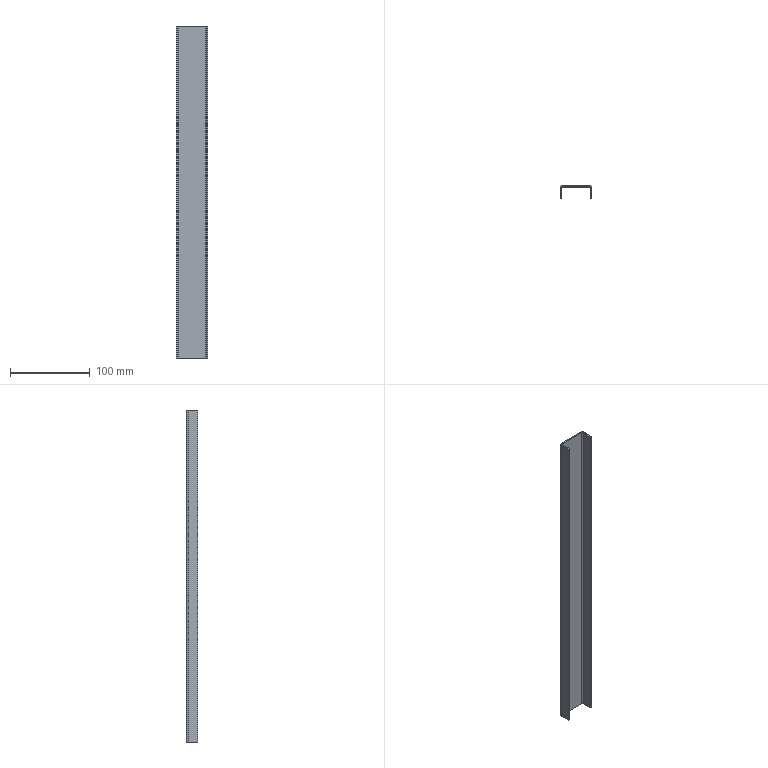Part | SolidWorks | features FlatPattern 1, SMBaseFlange 1, SheetMetal 1 | 1 solid | 22 faces | box 40 x 15 x 416 mm | volume 40603 mm3 | plane 18 | cylinder 4 | commonest cylinder face diameters 3 x2 6 x2
STEP:
#1=CARTESIAN_POINT('',(3.,15.,416.));
#2=VERTEX_POINT('',#1);
#3=CARTESIAN_POINT('',(3.,13.5,416.));
#4=VERTEX_POINT('',#3);
#5=CARTESIAN_POINT('',(3.,15.,416.));
#6=DIRECTION('',(0.,-1.,0.));
#7=VECTOR('',#6,1000.);
#8=LINE('',#5,#7);
#9=EDGE_CURVE('',#2,#4,#8,.T.);
#10=ORIENTED_EDGE('',*,*,#9,.F.);
#11=CARTESIAN_POINT('',(0.,12.,416.));
#12=VERTEX_POINT('',#11);
#13=CARTESIAN_POINT('',(3.,12.,416.));
#14=DIRECTION('',(0.,0.,-1.));
#15=DIRECTION('',(1.,0.,0.));
#16=AXIS2_PLACEMENT_3D('',#13,#14,#15);
#17=CIRCLE('',#16,3.);
#18=EDGE_CURVE('',#12,#2,#17,.T.);
#19=ORIENTED_EDGE('',*,*,#18,.F.);
#20=CARTESIAN_POINT('',(1.5,12.,416.));
#21=VERTEX_POINT('',#20);
#22=CARTESIAN_POINT('',(1.5,12.,416.));
#23=DIRECTION('',(-1.,0.,0.));
#24=VECTOR('',#23,1000.);
#25=LINE('',#22,#24);
#26=EDGE_CURVE('',#21,#12,#25,.T.);
#27=ORIENTED_EDGE('',*,*,#26,.F.);
#28=CARTESIAN_POINT('',(3.,12.,416.));
#29=DIRECTION('',(0.,0.,-1.));
#30=DIRECTION('',(1.,0.,0.));
#31=AXIS2_PLACEMENT_3D('',#28,#29,#30);
#32=CIRCLE('',#31,1.5);
#33=EDGE_CURVE('',#21,#4,#32,.T.);
#34=ORIENTED_EDGE('',*,*,#33,.T.);
#35=EDGE_LOOP('',(#10,#19,#27,#34));
#36=FACE_OUTER_BOUND('',#35,.T.);
#37=CARTESIAN_POINT('',(3.,15.,416.));
#38=DIRECTION('',(0.,0.,1.));
#39=DIRECTION('',(1.,0.,0.));
#40=AXIS2_PLACEMENT_3D('',#37,#38,#39);
#41=PLANE('',#40);
#42=ADVANCED_FACE('',(#36),#41,.T.);
#43=CARTESIAN_POINT('',(37.,15.,416.));
#44=VERTEX_POINT('',#43);
#45=CARTESIAN_POINT('',(0.,15.,416.));
#46=DIRECTION('',(1.,0.,0.));
#47=VECTOR('',#46,1000.);
#48=LINE('',#45,#47);
#49=EDGE_CURVE('',#2,#44,#48,.T.);
#50=ORIENTED_EDGE('',*,*,#49,.F.);
#51=ORIENTED_EDGE('',*,*,#9,.T.);
#52=CARTESIAN_POINT('',(37.,13.5,416.));
#53=VERTEX_POINT('',#52);
#54=CARTESIAN_POINT('',(0.,13.5,416.));
#55=DIRECTION('',(1.,0.,0.));
#56=VECTOR('',#55,1000.);
#57=LINE('',#54,#56);
#58=EDGE_CURVE('',#4,#53,#57,.T.);
#59=ORIENTED_EDGE('',*,*,#58,.T.);
#60=CARTESIAN_POINT('',(37.,13.5,416.));
#61=DIRECTION('',(0.,1.,0.));
#62=VECTOR('',#61,1000.);
#63=LINE('',#60,#62);
#64=EDGE_CURVE('',#53,#44,#63,.T.);
#65=ORIENTED_EDGE('',*,*,#64,.T.);
#66=EDGE_LOOP('',(#50,#51,#59,#65));
#67=FACE_OUTER_BOUND('',#66,.T.);
#68=CARTESIAN_POINT('',(1.5,12.,416.));
#69=DIRECTION('',(0.,0.,1.));
#70=DIRECTION('',(1.,0.,0.));
#71=AXIS2_PLACEMENT_3D('',#68,#69,#70);
#72=PLANE('',#71);
#73=ADVANCED_FACE('',(#67),#72,.T.);
#74=CARTESIAN_POINT('',(0.,12.,0.));
#75=VERTEX_POINT('',#74);
#76=CARTESIAN_POINT('',(1.5,12.,0.));
#77=VERTEX_POINT('',#76);
#78=CARTESIAN_POINT('',(0.,12.,0.));
#79=DIRECTION('',(1.,0.,0.));
#80=VECTOR('',#79,1000.);
#81=LINE('',#78,#80);
#82=EDGE_CURVE('',#75,#77,#81,.T.);
#83=ORIENTED_EDGE('',*,*,#82,.F.);
#84=CARTESIAN_POINT('',(3.,15.,0.));
#85=VERTEX_POINT('',#84);
#86=CARTESIAN_POINT('',(3.,12.,0.));
#87=DIRECTION('',(0.,0.,-1.));
#88=DIRECTION('',(1.,0.,0.));
#89=AXIS2_PLACEMENT_3D('',#86,#87,#88);
#90=CIRCLE('',#89,3.);
#91=EDGE_CURVE('',#75,#85,#90,.T.);
#92=ORIENTED_EDGE('',*,*,#91,.T.);
#93=CARTESIAN_POINT('',(3.,13.5,0.));
#94=VERTEX_POINT('',#93);
#95=CARTESIAN_POINT('',(3.,13.5,0.));
#96=DIRECTION('',(0.,1.,0.));
#97=VECTOR('',#96,1000.);
#98=LINE('',#95,#97);
#99=EDGE_CURVE('',#94,#85,#98,.T.);
#100=ORIENTED_EDGE('',*,*,#99,.F.);
#101=CARTESIAN_POINT('',(3.,12.,0.));
#102=DIRECTION('',(0.,0.,-1.));
#103=DIRECTION('',(1.,0.,0.));
#104=AXIS2_PLACEMENT_3D('',#101,#102,#103);
#105=CIRCLE('',#104,1.5);
#106=EDGE_CURVE('',#77,#94,#105,.T.);
#107=ORIENTED_EDGE('',*,*,#106,.F.);
#108=EDGE_LOOP('',(#83,#92,#100,#107));
#109=FACE_OUTER_BOUND('',#108,.T.);
#110=CARTESIAN_POINT('',(0.,12.,0.));
#111=DIRECTION('',(0.,0.,-1.));
#112=DIRECTION('',(-1.,0.,0.));
#113=AXIS2_PLACEMENT_3D('',#110,#111,#112);
#114=PLANE('',#113);
#115=ADVANCED_FACE('',(#109),#114,.T.);
#116=CARTESIAN_POINT('',(0.,0.,0.));
#117=VERTEX_POINT('',#116);
#118=CARTESIAN_POINT('',(0.,0.,0.));
#119=DIRECTION('',(0.,1.,0.));
#120=VECTOR('',#119,1000.);
#121=LINE('',#118,#120);
#122=EDGE_CURVE('',#117,#75,#121,.T.);
#123=ORIENTED_EDGE('',*,*,#122,.T.);
#124=ORIENTED_EDGE('',*,*,#82,.T.);
#125=CARTESIAN_POINT('',(1.5,0.,0.));
#126=VERTEX_POINT('',#125);
#127=CARTESIAN_POINT('',(1.5,0.,0.));
#128=DIRECTION('',(0.,1.,0.));
#129=VECTOR('',#128,1000.);
#130=LINE('',#127,#129);
#131=EDGE_CURVE('',#126,#77,#130,.T.);
#132=ORIENTED_EDGE('',*,*,#131,.F.);
#133=CARTESIAN_POINT('',(1.5,0.,0.));
#134=DIRECTION('',(-1.,0.,0.));
#135=VECTOR('',#134,1000.);
#136=LINE('',#133,#135);
#137=EDGE_CURVE('',#126,#117,#136,.T.);
#138=ORIENTED_EDGE('',*,*,#137,.T.);
#139=EDGE_LOOP('',(#123,#124,#132,#138));
#140=FACE_OUTER_BOUND('',#139,.T.);
#141=CARTESIAN_POINT('',(3.,13.5,0.));
#142=DIRECTION('',(0.,0.,-1.));
#143=DIRECTION('',(-1.,0.,0.));
#144=AXIS2_PLACEMENT_3D('',#141,#142,#143);
#145=PLANE('',#144);
#146=ADVANCED_FACE('',(#140),#145,.T.);
#147=CARTESIAN_POINT('',(40.,12.,416.));
#148=VERTEX_POINT('',#147);
#149=CARTESIAN_POINT('',(38.5,12.,416.));
#150=VERTEX_POINT('',#149);
#151=CARTESIAN_POINT('',(40.,12.,416.));
#152=DIRECTION('',(-1.,0.,0.));
#153=VECTOR('',#152,1000.);
#154=LINE('',#151,#153);
#155=EDGE_CURVE('',#148,#150,#154,.T.);
#156=ORIENTED_EDGE('',*,*,#155,.F.);
#157=CARTESIAN_POINT('',(37.,12.,416.));
#158=DIRECTION('',(0.,0.,-1.));
#159=DIRECTION('',(1.,0.,0.));
#160=AXIS2_PLACEMENT_3D('',#157,#158,#159);
#161=CIRCLE('',#160,3.);
#162=EDGE_CURVE('',#44,#148,#161,.T.);
#163=ORIENTED_EDGE('',*,*,#162,.F.);
#164=ORIENTED_EDGE('',*,*,#64,.F.);
#165=CARTESIAN_POINT('',(37.,12.,416.));
#166=DIRECTION('',(0.,0.,-1.));
#167=DIRECTION('',(1.,0.,0.));
#168=AXIS2_PLACEMENT_3D('',#165,#166,#167);
#169=CIRCLE('',#168,1.5);
#170=EDGE_CURVE('',#53,#150,#169,.T.);
#171=ORIENTED_EDGE('',*,*,#170,.T.);
#172=EDGE_LOOP('',(#156,#163,#164,#171));
#173=FACE_OUTER_BOUND('',#172,.T.);
#174=CARTESIAN_POINT('',(40.,12.,416.));
#175=DIRECTION('',(0.,0.,1.));
#176=DIRECTION('',(1.,0.,0.));
#177=AXIS2_PLACEMENT_3D('',#174,#175,#176);
#178=PLANE('',#177);
#179=ADVANCED_FACE('',(#173),#178,.T.);
#180=CARTESIAN_POINT('',(40.,0.,416.));
#181=VERTEX_POINT('',#180);
#182=CARTESIAN_POINT('',(40.,15.,416.));
#183=DIRECTION('',(0.,-1.,0.));
#184=VECTOR('',#183,1000.);
#185=LINE('',#182,#184);
#186=EDGE_CURVE('',#148,#181,#185,.T.);
#187=ORIENTED_EDGE('',*,*,#186,.F.);
#188=ORIENTED_EDGE('',*,*,#155,.T.);
#189=CARTESIAN_POINT('',(38.5,0.,416.));
#190=VERTEX_POINT('',#189);
#191=CARTESIAN_POINT('',(38.5,15.,416.));
#192=DIRECTION('',(0.,-1.,0.));
#193=VECTOR('',#192,1000.);
#194=LINE('',#191,#193);
#195=EDGE_CURVE('',#150,#190,#194,.T.);
#196=ORIENTED_EDGE('',*,*,#195,.T.);
#197=CARTESIAN_POINT('',(40.,0.,416.));
#198=DIRECTION('',(-1.,0.,0.));
#199=VECTOR('',#198,1000.);
#200=LINE('',#197,#199);
#201=EDGE_CURVE('',#181,#190,#200,.T.);
#202=ORIENTED_EDGE('',*,*,#201,.F.);
#203=EDGE_LOOP('',(#187,#188,#196,#202));
#204=FACE_OUTER_BOUND('',#203,.T.);
#205=CARTESIAN_POINT('',(37.,13.5,416.));
#206=DIRECTION('',(0.,0.,1.));
#207=DIRECTION('',(1.,0.,0.));
#208=AXIS2_PLACEMENT_3D('',#205,#206,#207);
#209=PLANE('',#208);
#210=ADVANCED_FACE('',(#204),#209,.T.);
#211=CARTESIAN_POINT('',(37.,15.,0.));
#212=VERTEX_POINT('',#211);
#213=CARTESIAN_POINT('',(37.,13.5,0.));
#214=VERTEX_POINT('',#213);
#215=CARTESIAN_POINT('',(37.,15.,0.));
#216=DIRECTION('',(0.,-1.,0.));
#217=VECTOR('',#216,1000.);
#218=LINE('',#215,#217);
#219=EDGE_CURVE('',#212,#214,#218,.T.);
#220=ORIENTED_EDGE('',*,*,#219,.F.);
#221=CARTESIAN_POINT('',(40.,12.,0.));
#222=VERTEX_POINT('',#221);
#223=CARTESIAN_POINT('',(37.,12.,0.));
#224=DIRECTION('',(0.,0.,-1.));
#225=DIRECTION('',(1.,0.,0.));
#226=AXIS2_PLACEMENT_3D('',#223,#224,#225);
#227=CIRCLE('',#226,3.);
#228=EDGE_CURVE('',#212,#222,#227,.T.);
#229=ORIENTED_EDGE('',*,*,#228,.T.);
#230=CARTESIAN_POINT('',(38.5,12.,0.));
#231=VERTEX_POINT('',#230);
#232=CARTESIAN_POINT('',(38.5,12.,0.));
#233=DIRECTION('',(1.,0.,0.));
#234=VECTOR('',#233,1000.);
#235=LINE('',#232,#234);
#236=EDGE_CURVE('',#231,#222,#235,.T.);
#237=ORIENTED_EDGE('',*,*,#236,.F.);
#238=CARTESIAN_POINT('',(37.,12.,0.));
#239=DIRECTION('',(0.,0.,-1.));
#240=DIRECTION('',(1.,0.,0.));
#241=AXIS2_PLACEMENT_3D('',#238,#239,#240);
#242=CIRCLE('',#241,1.5);
#243=EDGE_CURVE('',#214,#231,#242,.T.);
#244=ORIENTED_EDGE('',*,*,#243,.F.);
#245=EDGE_LOOP('',(#220,#229,#237,#244));
#246=FACE_OUTER_BOUND('',#245,.T.);
#247=CARTESIAN_POINT('',(37.,15.,0.));
#248=DIRECTION('',(0.,0.,-1.));
#249=DIRECTION('',(-1.,0.,0.));
#250=AXIS2_PLACEMENT_3D('',#247,#248,#249);
#251=PLANE('',#250);
#252=ADVANCED_FACE('',(#246),#251,.T.);
#253=CARTESIAN_POINT('',(0.,15.,0.));
#254=DIRECTION('',(1.,0.,0.));
#255=VECTOR('',#254,1000.);
#256=LINE('',#253,#255);
#257=EDGE_CURVE('',#85,#212,#256,.T.);
#258=ORIENTED_EDGE('',*,*,#257,.T.);
#259=ORIENTED_EDGE('',*,*,#219,.T.);
#260=CARTESIAN_POINT('',(0.,13.5,0.));
#261=DIRECTION('',(1.,0.,0.));
#262=VECTOR('',#261,1000.);
#263=LINE('',#260,#262);
#264=EDGE_CURVE('',#94,#214,#263,.T.);
#265=ORIENTED_EDGE('',*,*,#264,.F.);
#266=ORIENTED_EDGE('',*,*,#99,.T.);
#267=EDGE_LOOP('',(#258,#259,#265,#266));
#268=FACE_OUTER_BOUND('',#267,.T.);
#269=CARTESIAN_POINT('',(38.5,12.,0.));
#270=DIRECTION('',(0.,0.,-1.));
#271=DIRECTION('',(-1.,0.,0.));
#272=AXIS2_PLACEMENT_3D('',#269,#270,#271);
#273=PLANE('',#272);
#274=ADVANCED_FACE('',(#268),#273,.T.);
#275=CARTESIAN_POINT('',(38.5,0.,0.));
#276=VERTEX_POINT('',#275);
#277=CARTESIAN_POINT('',(38.5,15.,0.));
#278=DIRECTION('',(0.,-1.,0.));
#279=VECTOR('',#278,1000.);
#280=LINE('',#277,#279);
#281=EDGE_CURVE('',#231,#276,#280,.T.);
#282=ORIENTED_EDGE('',*,*,#281,.T.);
#283=CARTESIAN_POINT('',(38.5,0.,416.));
#284=DIRECTION('',(0.,0.,-1.));
#285=VECTOR('',#284,1000.);
#286=LINE('',#283,#285);
#287=EDGE_CURVE('',#190,#276,#286,.T.);
#288=ORIENTED_EDGE('',*,*,#287,.F.);
#289=ORIENTED_EDGE('',*,*,#195,.F.);
#290=CARTESIAN_POINT('',(38.5,12.,416.));
#291=DIRECTION('',(0.,0.,-1.));
#292=VECTOR('',#291,1000.);
#293=LINE('',#290,#292);
#294=EDGE_CURVE('',#150,#231,#293,.T.);
#295=ORIENTED_EDGE('',*,*,#294,.T.);
#296=EDGE_LOOP('',(#282,#288,#289,#295));
#297=FACE_OUTER_BOUND('',#296,.T.);
#298=CARTESIAN_POINT('',(38.5,15.,416.));
#299=DIRECTION('',(1.,0.,0.));
#300=DIRECTION('',(0.,1.,0.));
#301=AXIS2_PLACEMENT_3D('',#298,#299,#300);
#302=PLANE('',#301);
#303=ADVANCED_FACE('',(#297),#302,.F.);
#304=CARTESIAN_POINT('',(40.,0.,0.));
#305=VERTEX_POINT('',#304);
#306=CARTESIAN_POINT('',(40.,0.,0.));
#307=DIRECTION('',(-1.,0.,0.));
#308=VECTOR('',#307,1000.);
#309=LINE('',#306,#308);
#310=EDGE_CURVE('',#305,#276,#309,.T.);
#311=ORIENTED_EDGE('',*,*,#310,.F.);
#312=CARTESIAN_POINT('',(40.,0.,416.));
#313=DIRECTION('',(0.,0.,-1.));
#314=VECTOR('',#313,1000.);
#315=LINE('',#312,#314);
#316=EDGE_CURVE('',#181,#305,#315,.T.);
#317=ORIENTED_EDGE('',*,*,#316,.F.);
#318=ORIENTED_EDGE('',*,*,#201,.T.);
#319=ORIENTED_EDGE('',*,*,#287,.T.);
#320=EDGE_LOOP('',(#311,#317,#318,#319));
#321=FACE_OUTER_BOUND('',#320,.T.);
#322=CARTESIAN_POINT('',(40.,0.,416.));
#323=DIRECTION('',(0.,-1.,0.));
#324=DIRECTION('',(0.,0.,-1.));
#325=AXIS2_PLACEMENT_3D('',#322,#323,#324);
#326=PLANE('',#325);
#327=ADVANCED_FACE('',(#321),#326,.T.);
#328=CARTESIAN_POINT('',(40.,15.,0.));
#329=DIRECTION('',(0.,-1.,0.));
#330=VECTOR('',#329,1000.);
#331=LINE('',#328,#330);
#332=EDGE_CURVE('',#222,#305,#331,.T.);
#333=ORIENTED_EDGE('',*,*,#332,.F.);
#334=CARTESIAN_POINT('',(40.,12.,416.));
#335=DIRECTION('',(0.,0.,-1.));
#336=VECTOR('',#335,1000.);
#337=LINE('',#334,#336);
#338=EDGE_CURVE('',#148,#222,#337,.T.);
#339=ORIENTED_EDGE('',*,*,#338,.F.);
#340=ORIENTED_EDGE('',*,*,#186,.T.);
#341=ORIENTED_EDGE('',*,*,#316,.T.);
#342=EDGE_LOOP('',(#333,#339,#340,#341));
#343=FACE_OUTER_BOUND('',#342,.T.);
#344=CARTESIAN_POINT('',(40.,15.,416.));
#345=DIRECTION('',(1.,0.,0.));
#346=DIRECTION('',(0.,1.,0.));
#347=AXIS2_PLACEMENT_3D('',#344,#345,#346);
#348=PLANE('',#347);
#349=ADVANCED_FACE('',(#343),#348,.T.);
#350=ORIENTED_EDGE('',*,*,#228,.F.);
#351=CARTESIAN_POINT('',(37.,15.,416.));
#352=DIRECTION('',(0.,0.,-1.));
#353=VECTOR('',#352,1000.);
#354=LINE('',#351,#353);
#355=EDGE_CURVE('',#44,#212,#354,.T.);
#356=ORIENTED_EDGE('',*,*,#355,.F.);
#357=ORIENTED_EDGE('',*,*,#162,.T.);
#358=ORIENTED_EDGE('',*,*,#338,.T.);
#359=EDGE_LOOP('',(#350,#356,#357,#358));
#360=FACE_OUTER_BOUND('',#359,.T.);
#361=CARTESIAN_POINT('',(37.,12.,416.));
#362=DIRECTION('',(0.,0.,-1.));
#363=DIRECTION('',(-1.,0.,0.));
#364=AXIS2_PLACEMENT_3D('',#361,#362,#363);
#365=CYLINDRICAL_SURFACE('',#364,3.);
#366=ADVANCED_FACE('',(#360),#365,.T.);
#367=ORIENTED_EDGE('',*,*,#257,.F.);
#368=CARTESIAN_POINT('',(3.,15.,416.));
#369=DIRECTION('',(0.,0.,-1.));
#370=VECTOR('',#369,1000.);
#371=LINE('',#368,#370);
#372=EDGE_CURVE('',#2,#85,#371,.T.);
#373=ORIENTED_EDGE('',*,*,#372,.F.);
#374=ORIENTED_EDGE('',*,*,#49,.T.);
#375=ORIENTED_EDGE('',*,*,#355,.T.);
#376=EDGE_LOOP('',(#367,#373,#374,#375));
#377=FACE_OUTER_BOUND('',#376,.T.);
#378=CARTESIAN_POINT('',(0.,15.,416.));
#379=DIRECTION('',(0.,1.,0.));
#380=DIRECTION('',(0.,0.,1.));
#381=AXIS2_PLACEMENT_3D('',#378,#379,#380);
#382=PLANE('',#381);
#383=ADVANCED_FACE('',(#377),#382,.T.);
#384=ORIENTED_EDGE('',*,*,#91,.F.);
#385=CARTESIAN_POINT('',(0.,12.,416.));
#386=DIRECTION('',(0.,0.,-1.));
#387=VECTOR('',#386,1000.);
#388=LINE('',#385,#387);
#389=EDGE_CURVE('',#12,#75,#388,.T.);
#390=ORIENTED_EDGE('',*,*,#389,.F.);
#391=ORIENTED_EDGE('',*,*,#18,.T.);
#392=ORIENTED_EDGE('',*,*,#372,.T.);
#393=EDGE_LOOP('',(#384,#390,#391,#392));
#394=FACE_OUTER_BOUND('',#393,.T.);
#395=CARTESIAN_POINT('',(3.,12.,416.));
#396=DIRECTION('',(0.,0.,-1.));
#397=DIRECTION('',(-1.,0.,0.));
#398=AXIS2_PLACEMENT_3D('',#395,#396,#397);
#399=CYLINDRICAL_SURFACE('',#398,3.);
#400=ADVANCED_FACE('',(#394),#399,.T.);
#401=ORIENTED_EDGE('',*,*,#122,.F.);
#402=CARTESIAN_POINT('',(0.,0.,416.));
#403=VERTEX_POINT('',#402);
#404=CARTESIAN_POINT('',(0.,0.,416.));
#405=DIRECTION('',(0.,0.,-1.));
#406=VECTOR('',#405,1000.);
#407=LINE('',#404,#406);
#408=EDGE_CURVE('',#403,#117,#407,.T.);
#409=ORIENTED_EDGE('',*,*,#408,.F.);
#410=CARTESIAN_POINT('',(0.,0.,416.));
#411=DIRECTION('',(0.,1.,0.));
#412=VECTOR('',#411,1000.);
#413=LINE('',#410,#412);
#414=EDGE_CURVE('',#403,#12,#413,.T.);
#415=ORIENTED_EDGE('',*,*,#414,.T.);
#416=ORIENTED_EDGE('',*,*,#389,.T.);
#417=EDGE_LOOP('',(#401,#409,#415,#416));
#418=FACE_OUTER_BOUND('',#417,.T.);
#419=CARTESIAN_POINT('',(0.,0.,416.));
#420=DIRECTION('',(-1.,0.,0.));
#421=DIRECTION('',(0.,0.,1.));
#422=AXIS2_PLACEMENT_3D('',#419,#420,#421);
#423=PLANE('',#422);
#424=ADVANCED_FACE('',(#418),#423,.T.);
#425=ORIENTED_EDGE('',*,*,#137,.F.);
#426=CARTESIAN_POINT('',(1.5,0.,416.));
#427=VERTEX_POINT('',#426);
#428=CARTESIAN_POINT('',(1.5,0.,416.));
#429=DIRECTION('',(0.,0.,-1.));
#430=VECTOR('',#429,1000.);
#431=LINE('',#428,#430);
#432=EDGE_CURVE('',#427,#126,#431,.T.);
#433=ORIENTED_EDGE('',*,*,#432,.F.);
#434=CARTESIAN_POINT('',(1.5,0.,416.));
#435=DIRECTION('',(-1.,0.,0.));
#436=VECTOR('',#435,1000.);
#437=LINE('',#434,#436);
#438=EDGE_CURVE('',#427,#403,#437,.T.);
#439=ORIENTED_EDGE('',*,*,#438,.T.);
#440=ORIENTED_EDGE('',*,*,#408,.T.);
#441=EDGE_LOOP('',(#425,#433,#439,#440));
#442=FACE_OUTER_BOUND('',#441,.T.);
#443=CARTESIAN_POINT('',(1.5,0.,416.));
#444=DIRECTION('',(0.,-1.,0.));
#445=DIRECTION('',(0.,0.,-1.));
#446=AXIS2_PLACEMENT_3D('',#443,#444,#445);
#447=PLANE('',#446);
#448=ADVANCED_FACE('',(#442),#447,.T.);
#449=ORIENTED_EDGE('',*,*,#131,.T.);
#450=CARTESIAN_POINT('',(1.5,12.,416.));
#451=DIRECTION('',(0.,0.,-1.));
#452=VECTOR('',#451,1000.);
#453=LINE('',#450,#452);
#454=EDGE_CURVE('',#21,#77,#453,.T.);
#455=ORIENTED_EDGE('',*,*,#454,.F.);
#456=CARTESIAN_POINT('',(1.5,0.,416.));
#457=DIRECTION('',(0.,1.,0.));
#458=VECTOR('',#457,1000.);
#459=LINE('',#456,#458);
#460=EDGE_CURVE('',#427,#21,#459,.T.);
#461=ORIENTED_EDGE('',*,*,#460,.F.);
#462=ORIENTED_EDGE('',*,*,#432,.T.);
#463=EDGE_LOOP('',(#449,#455,#461,#462));
#464=FACE_OUTER_BOUND('',#463,.T.);
#465=CARTESIAN_POINT('',(1.5,0.,416.));
#466=DIRECTION('',(-1.,0.,0.));
#467=DIRECTION('',(0.,0.,1.));
#468=AXIS2_PLACEMENT_3D('',#465,#466,#467);
#469=PLANE('',#468);
#470=ADVANCED_FACE('',(#464),#469,.F.);
#471=ORIENTED_EDGE('',*,*,#106,.T.);
#472=CARTESIAN_POINT('',(3.,13.5,416.));
#473=DIRECTION('',(0.,0.,-1.));
#474=VECTOR('',#473,1000.);
#475=LINE('',#472,#474);
#476=EDGE_CURVE('',#4,#94,#475,.T.);
#477=ORIENTED_EDGE('',*,*,#476,.F.);
#478=ORIENTED_EDGE('',*,*,#33,.F.);
#479=ORIENTED_EDGE('',*,*,#454,.T.);
#480=EDGE_LOOP('',(#471,#477,#478,#479));
#481=FACE_OUTER_BOUND('',#480,.T.);
#482=CARTESIAN_POINT('',(3.,12.,416.));
#483=DIRECTION('',(0.,0.,-1.));
#484=DIRECTION('',(-1.,0.,0.));
#485=AXIS2_PLACEMENT_3D('',#482,#483,#484);
#486=CYLINDRICAL_SURFACE('',#485,1.5);
#487=ADVANCED_FACE('',(#481),#486,.F.);
#488=ORIENTED_EDGE('',*,*,#264,.T.);
#489=CARTESIAN_POINT('',(37.,13.5,416.));
#490=DIRECTION('',(0.,0.,-1.));
#491=VECTOR('',#490,1000.);
#492=LINE('',#489,#491);
#493=EDGE_CURVE('',#53,#214,#492,.T.);
#494=ORIENTED_EDGE('',*,*,#493,.F.);
#495=ORIENTED_EDGE('',*,*,#58,.F.);
#496=ORIENTED_EDGE('',*,*,#476,.T.);
#497=EDGE_LOOP('',(#488,#494,#495,#496));
#498=FACE_OUTER_BOUND('',#497,.T.);
#499=CARTESIAN_POINT('',(0.,13.5,416.));
#500=DIRECTION('',(0.,1.,0.));
#501=DIRECTION('',(0.,0.,1.));
#502=AXIS2_PLACEMENT_3D('',#499,#500,#501);
#503=PLANE('',#502);
#504=ADVANCED_FACE('',(#498),#503,.F.);
#505=ORIENTED_EDGE('',*,*,#243,.T.);
#506=ORIENTED_EDGE('',*,*,#294,.F.);
#507=ORIENTED_EDGE('',*,*,#170,.F.);
#508=ORIENTED_EDGE('',*,*,#493,.T.);
#509=EDGE_LOOP('',(#505,#506,#507,#508));
#510=FACE_OUTER_BOUND('',#509,.T.);
#511=CARTESIAN_POINT('',(37.,12.,416.));
#512=DIRECTION('',(0.,0.,-1.));
#513=DIRECTION('',(-1.,0.,0.));
#514=AXIS2_PLACEMENT_3D('',#511,#512,#513);
#515=CYLINDRICAL_SURFACE('',#514,1.5);
#516=ADVANCED_FACE('',(#510),#515,.F.);
#517=ORIENTED_EDGE('',*,*,#460,.T.);
#518=ORIENTED_EDGE('',*,*,#26,.T.);
#519=ORIENTED_EDGE('',*,*,#414,.F.);
#520=ORIENTED_EDGE('',*,*,#438,.F.);
#521=EDGE_LOOP('',(#517,#518,#519,#520));
#522=FACE_OUTER_BOUND('',#521,.T.);
#523=CARTESIAN_POINT('',(37.,12.,416.));
#524=DIRECTION('',(0.,0.,1.));
#525=DIRECTION('',(1.,0.,0.));
#526=AXIS2_PLACEMENT_3D('',#523,#524,#525);
#527=PLANE('',#526);
#528=ADVANCED_FACE('',(#522),#527,.T.);
#529=ORIENTED_EDGE('',*,*,#281,.F.);
#530=ORIENTED_EDGE('',*,*,#236,.T.);
#531=ORIENTED_EDGE('',*,*,#332,.T.);
#532=ORIENTED_EDGE('',*,*,#310,.T.);
#533=EDGE_LOOP('',(#529,#530,#531,#532));
#534=FACE_OUTER_BOUND('',#533,.T.);
#535=CARTESIAN_POINT('',(37.,12.,0.));
#536=DIRECTION('',(0.,0.,1.));
#537=DIRECTION('',(1.,0.,0.));
#538=AXIS2_PLACEMENT_3D('',#535,#536,#537);
#539=PLANE('',#538);
#540=ADVANCED_FACE('',(#534),#539,.F.);
#541=CLOSED_SHELL('',(#42,#73,#115,#146,#179,#210,#252,#274,#303,#327,#349,#366,#383,#400,#424,#448,#470,#487,#504,#516,#528,#540));
#542=MANIFOLD_SOLID_BREP('',#541);
#543=CARTESIAN_POINT('',(0.,0.,0.));
#544=DIRECTION('',(0.,0.,1.));
#545=DIRECTION('',(1.,0.,0.));
#546=AXIS2_PLACEMENT_3D('',#543,#544,#545);
#547=(LENGTH_UNIT()NAMED_UNIT(*)SI_UNIT(.MILLI.,.METRE.));
#548=UNCERTAINTY_MEASURE_WITH_UNIT(LENGTH_MEASURE(0.00001),#547,'','');
#549=(NAMED_UNIT(*)PLANE_ANGLE_UNIT()SI_UNIT($,.RADIAN.));
#550=(NAMED_UNIT(*)SI_UNIT($,.STERADIAN.)SOLID_ANGLE_UNIT());
#551=(GEOMETRIC_REPRESENTATION_CONTEXT(3)GLOBAL_UNCERTAINTY_ASSIGNED_CONTEXT((#548))GLOBAL_UNIT_ASSIGNED_CONTEXT((#547,#549,#550))REPRESENTATION_CONTEXT('',''));
#552=ADVANCED_BREP_SHAPE_REPRESENTATION('',(#542,#546),#551);